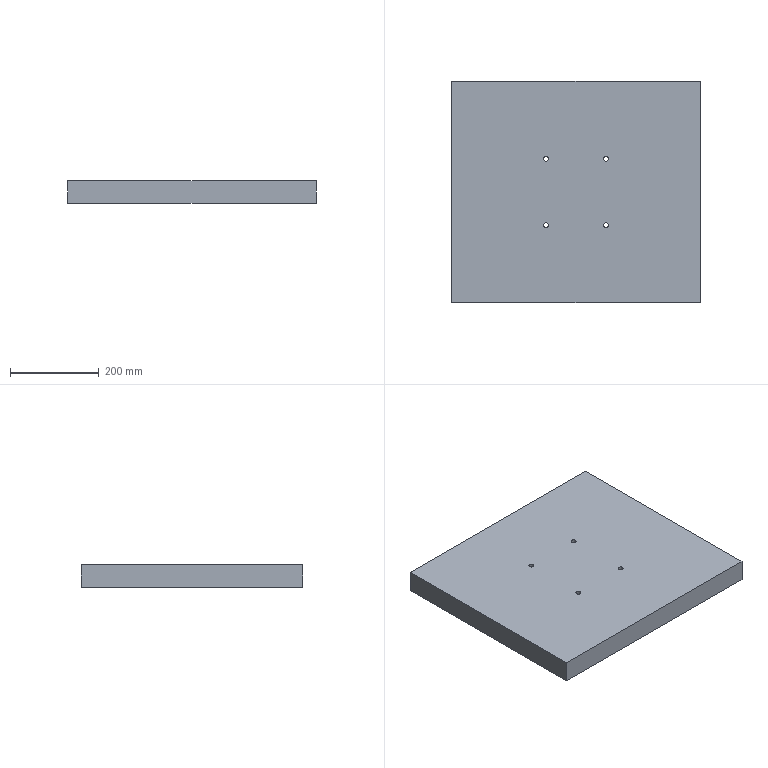Part | SolidWorks | features Extrusion 1, HoleWzd 1, ICE 1 | 1 solid | 22 faces | box 560 x 500 x 50 mm | volume 13976046 mm3 | cylinder 12 | plane 6 | cone 4 | commonest cylinder face diameters 11 x8 10.2 x4
STEP:
#1=CARTESIAN_POINT('',(-73.,-75.,0.));
#2=VERTEX_POINT('',#1);
#3=CARTESIAN_POINT('',(-62.,-75.,0.));
#4=VERTEX_POINT('',#3);
#5=CARTESIAN_POINT('',(-67.5,-75.,0.));
#6=DIRECTION('',(0.,0.,1.));
#7=DIRECTION('',(1.,0.,0.));
#8=AXIS2_PLACEMENT_3D('',#5,#6,#7);
#9=CIRCLE('',#8,5.5);
#10=EDGE_CURVE('',#2,#4,#9,.T.);
#11=ORIENTED_EDGE('',*,*,#10,.F.);
#12=CARTESIAN_POINT('',(-73.,-75.,50.));
#13=VERTEX_POINT('',#12);
#14=CARTESIAN_POINT('',(-73.,-75.,0.));
#15=DIRECTION('',(0.,0.,1.));
#16=VECTOR('',#15,1000.);
#17=LINE('',#14,#16);
#18=EDGE_CURVE('',#2,#13,#17,.T.);
#19=ORIENTED_EDGE('',*,*,#18,.T.);
#20=CARTESIAN_POINT('',(-62.,-75.,50.));
#21=VERTEX_POINT('',#20);
#22=CARTESIAN_POINT('',(-67.5,-75.,50.));
#23=DIRECTION('',(0.,0.,1.));
#24=DIRECTION('',(1.,0.,0.));
#25=AXIS2_PLACEMENT_3D('',#22,#23,#24);
#26=CIRCLE('',#25,5.5);
#27=EDGE_CURVE('',#13,#21,#26,.T.);
#28=ORIENTED_EDGE('',*,*,#27,.T.);
#29=CARTESIAN_POINT('',(-62.,-75.,0.));
#30=DIRECTION('',(0.,0.,1.));
#31=VECTOR('',#30,1000.);
#32=LINE('',#29,#31);
#33=EDGE_CURVE('',#4,#21,#32,.T.);
#34=ORIENTED_EDGE('',*,*,#33,.F.);
#35=EDGE_LOOP('',(#11,#19,#28,#34));
#36=FACE_OUTER_BOUND('',#35,.T.);
#37=CARTESIAN_POINT('',(-67.5,-75.,0.));
#38=DIRECTION('',(0.,0.,1.));
#39=DIRECTION('',(1.,0.,0.));
#40=AXIS2_PLACEMENT_3D('',#37,#38,#39);
#41=CYLINDRICAL_SURFACE('',#40,5.5);
#42=ADVANCED_FACE('',(#36),#41,.F.);
#43=CARTESIAN_POINT('',(62.,-75.,0.));
#44=VERTEX_POINT('',#43);
#45=CARTESIAN_POINT('',(73.,-75.,0.));
#46=VERTEX_POINT('',#45);
#47=CARTESIAN_POINT('',(67.5,-75.,0.));
#48=DIRECTION('',(0.,0.,1.));
#49=DIRECTION('',(1.,0.,0.));
#50=AXIS2_PLACEMENT_3D('',#47,#48,#49);
#51=CIRCLE('',#50,5.5);
#52=EDGE_CURVE('',#44,#46,#51,.T.);
#53=ORIENTED_EDGE('',*,*,#52,.F.);
#54=CARTESIAN_POINT('',(62.,-75.,50.));
#55=VERTEX_POINT('',#54);
#56=CARTESIAN_POINT('',(62.,-75.,0.));
#57=DIRECTION('',(0.,0.,1.));
#58=VECTOR('',#57,1000.);
#59=LINE('',#56,#58);
#60=EDGE_CURVE('',#44,#55,#59,.T.);
#61=ORIENTED_EDGE('',*,*,#60,.T.);
#62=CARTESIAN_POINT('',(73.,-75.,50.));
#63=VERTEX_POINT('',#62);
#64=CARTESIAN_POINT('',(67.5,-75.,50.));
#65=DIRECTION('',(0.,0.,1.));
#66=DIRECTION('',(1.,0.,0.));
#67=AXIS2_PLACEMENT_3D('',#64,#65,#66);
#68=CIRCLE('',#67,5.5);
#69=EDGE_CURVE('',#55,#63,#68,.T.);
#70=ORIENTED_EDGE('',*,*,#69,.T.);
#71=CARTESIAN_POINT('',(73.,-75.,0.));
#72=DIRECTION('',(0.,0.,1.));
#73=VECTOR('',#72,1000.);
#74=LINE('',#71,#73);
#75=EDGE_CURVE('',#46,#63,#74,.T.);
#76=ORIENTED_EDGE('',*,*,#75,.F.);
#77=EDGE_LOOP('',(#53,#61,#70,#76));
#78=FACE_OUTER_BOUND('',#77,.T.);
#79=CARTESIAN_POINT('',(67.5,-75.,0.));
#80=DIRECTION('',(0.,0.,1.));
#81=DIRECTION('',(1.,0.,0.));
#82=AXIS2_PLACEMENT_3D('',#79,#80,#81);
#83=CYLINDRICAL_SURFACE('',#82,5.5);
#84=ADVANCED_FACE('',(#78),#83,.F.);
#85=CARTESIAN_POINT('',(62.,75.,0.));
#86=VERTEX_POINT('',#85);
#87=CARTESIAN_POINT('',(73.,75.,0.));
#88=VERTEX_POINT('',#87);
#89=CARTESIAN_POINT('',(67.5,75.,0.));
#90=DIRECTION('',(0.,0.,1.));
#91=DIRECTION('',(1.,0.,0.));
#92=AXIS2_PLACEMENT_3D('',#89,#90,#91);
#93=CIRCLE('',#92,5.5);
#94=EDGE_CURVE('',#86,#88,#93,.T.);
#95=ORIENTED_EDGE('',*,*,#94,.F.);
#96=CARTESIAN_POINT('',(62.,75.,50.));
#97=VERTEX_POINT('',#96);
#98=CARTESIAN_POINT('',(62.,75.,0.));
#99=DIRECTION('',(0.,0.,1.));
#100=VECTOR('',#99,1000.);
#101=LINE('',#98,#100);
#102=EDGE_CURVE('',#86,#97,#101,.T.);
#103=ORIENTED_EDGE('',*,*,#102,.T.);
#104=CARTESIAN_POINT('',(73.,75.,50.));
#105=VERTEX_POINT('',#104);
#106=CARTESIAN_POINT('',(67.5,75.,50.));
#107=DIRECTION('',(0.,0.,1.));
#108=DIRECTION('',(1.,0.,0.));
#109=AXIS2_PLACEMENT_3D('',#106,#107,#108);
#110=CIRCLE('',#109,5.5);
#111=EDGE_CURVE('',#97,#105,#110,.T.);
#112=ORIENTED_EDGE('',*,*,#111,.T.);
#113=CARTESIAN_POINT('',(73.,75.,0.));
#114=DIRECTION('',(0.,0.,1.));
#115=VECTOR('',#114,1000.);
#116=LINE('',#113,#115);
#117=EDGE_CURVE('',#88,#105,#116,.T.);
#118=ORIENTED_EDGE('',*,*,#117,.F.);
#119=EDGE_LOOP('',(#95,#103,#112,#118));
#120=FACE_OUTER_BOUND('',#119,.T.);
#121=CARTESIAN_POINT('',(67.5,75.,0.));
#122=DIRECTION('',(0.,0.,1.));
#123=DIRECTION('',(1.,0.,0.));
#124=AXIS2_PLACEMENT_3D('',#121,#122,#123);
#125=CYLINDRICAL_SURFACE('',#124,5.5);
#126=ADVANCED_FACE('',(#120),#125,.F.);
#127=CARTESIAN_POINT('',(-73.,75.,0.));
#128=VERTEX_POINT('',#127);
#129=CARTESIAN_POINT('',(-62.,75.,0.));
#130=VERTEX_POINT('',#129);
#131=CARTESIAN_POINT('',(-67.5,75.,0.));
#132=DIRECTION('',(0.,0.,1.));
#133=DIRECTION('',(1.,0.,0.));
#134=AXIS2_PLACEMENT_3D('',#131,#132,#133);
#135=CIRCLE('',#134,5.5);
#136=EDGE_CURVE('',#128,#130,#135,.T.);
#137=ORIENTED_EDGE('',*,*,#136,.F.);
#138=CARTESIAN_POINT('',(-73.,75.,50.));
#139=VERTEX_POINT('',#138);
#140=CARTESIAN_POINT('',(-73.,75.,0.));
#141=DIRECTION('',(0.,0.,1.));
#142=VECTOR('',#141,1000.);
#143=LINE('',#140,#142);
#144=EDGE_CURVE('',#128,#139,#143,.T.);
#145=ORIENTED_EDGE('',*,*,#144,.T.);
#146=CARTESIAN_POINT('',(-62.,75.,50.));
#147=VERTEX_POINT('',#146);
#148=CARTESIAN_POINT('',(-67.5,75.,50.));
#149=DIRECTION('',(0.,0.,1.));
#150=DIRECTION('',(1.,0.,0.));
#151=AXIS2_PLACEMENT_3D('',#148,#149,#150);
#152=CIRCLE('',#151,5.5);
#153=EDGE_CURVE('',#139,#147,#152,.T.);
#154=ORIENTED_EDGE('',*,*,#153,.T.);
#155=CARTESIAN_POINT('',(-62.,75.,0.));
#156=DIRECTION('',(0.,0.,1.));
#157=VECTOR('',#156,1000.);
#158=LINE('',#155,#157);
#159=EDGE_CURVE('',#130,#147,#158,.T.);
#160=ORIENTED_EDGE('',*,*,#159,.F.);
#161=EDGE_LOOP('',(#137,#145,#154,#160));
#162=FACE_OUTER_BOUND('',#161,.T.);
#163=CARTESIAN_POINT('',(-67.5,75.,0.));
#164=DIRECTION('',(0.,0.,1.));
#165=DIRECTION('',(1.,0.,0.));
#166=AXIS2_PLACEMENT_3D('',#163,#164,#165);
#167=CYLINDRICAL_SURFACE('',#166,5.5);
#168=ADVANCED_FACE('',(#162),#167,.F.);
#169=CARTESIAN_POINT('',(-160.,220.75,19.9));
#170=VERTEX_POINT('',#169);
#171=CARTESIAN_POINT('',(-160.,220.75,30.1));
#172=VERTEX_POINT('',#171);
#173=CARTESIAN_POINT('',(-160.,220.75,25.));
#174=DIRECTION('',(0.,1.,0.));
#175=DIRECTION('',(0.,0.,1.));
#176=AXIS2_PLACEMENT_3D('',#173,#174,#175);
#177=CIRCLE('',#176,5.1);
#178=EDGE_CURVE('',#170,#172,#177,.T.);
#179=ORIENTED_EDGE('',*,*,#178,.F.);
#180=CARTESIAN_POINT('',(-160.,250.,19.9));
#181=VERTEX_POINT('',#180);
#182=CARTESIAN_POINT('',(-160.,250.,19.9));
#183=DIRECTION('',(0.,1.,0.));
#184=VECTOR('',#183,1000.);
#185=LINE('',#182,#184);
#186=EDGE_CURVE('',#170,#181,#185,.T.);
#187=ORIENTED_EDGE('',*,*,#186,.T.);
#188=CARTESIAN_POINT('',(-160.,250.,30.1));
#189=VERTEX_POINT('',#188);
#190=CARTESIAN_POINT('',(-160.,250.,25.));
#191=DIRECTION('',(0.,1.,0.));
#192=DIRECTION('',(0.,0.,1.));
#193=AXIS2_PLACEMENT_3D('',#190,#191,#192);
#194=CIRCLE('',#193,5.1);
#195=EDGE_CURVE('',#181,#189,#194,.T.);
#196=ORIENTED_EDGE('',*,*,#195,.T.);
#197=CARTESIAN_POINT('',(-160.,250.,30.1));
#198=DIRECTION('',(0.,1.,0.));
#199=VECTOR('',#198,1000.);
#200=LINE('',#197,#199);
#201=EDGE_CURVE('',#172,#189,#200,.T.);
#202=ORIENTED_EDGE('',*,*,#201,.F.);
#203=EDGE_LOOP('',(#179,#187,#196,#202));
#204=FACE_OUTER_BOUND('',#203,.T.);
#205=CARTESIAN_POINT('',(-160.,250.,25.));
#206=DIRECTION('',(0.,1.,0.));
#207=DIRECTION('',(0.,0.,1.));
#208=AXIS2_PLACEMENT_3D('',#205,#206,#207);
#209=CYLINDRICAL_SURFACE('',#208,5.1);
#210=ADVANCED_FACE('',(#204),#209,.F.);
#211=CARTESIAN_POINT('',(-160.,217.686,25.));
#212=VERTEX_POINT('',#211);
#213=CARTESIAN_POINT('',(-160.,220.75,30.1));
#214=DIRECTION('',(0.,0.515,0.8572));
#215=VECTOR('',#214,1000.);
#216=LINE('',#213,#215);
#217=EDGE_CURVE('',#212,#172,#216,.T.);
#218=ORIENTED_EDGE('',*,*,#217,.F.);
#219=CARTESIAN_POINT('',(-160.,220.75,19.9));
#220=DIRECTION('',(0.,0.515,-0.8572));
#221=VECTOR('',#220,1000.);
#222=LINE('',#219,#221);
#223=EDGE_CURVE('',#212,#170,#222,.T.);
#224=ORIENTED_EDGE('',*,*,#223,.T.);
#225=ORIENTED_EDGE('',*,*,#178,.T.);
#226=EDGE_LOOP('',(#218,#224,#225));
#227=FACE_OUTER_BOUND('',#226,.T.);
#228=CARTESIAN_POINT('',(-160.,220.75,25.));
#229=DIRECTION('',(0.,1.,0.));
#230=DIRECTION('',(0.,0.,1.));
#231=AXIS2_PLACEMENT_3D('',#228,#229,#230);
#232=CONICAL_SURFACE('',#231,5.1,1.03);
#233=ADVANCED_FACE('',(#227),#232,.F.);
#234=CARTESIAN_POINT('',(160.,220.75,19.9));
#235=VERTEX_POINT('',#234);
#236=CARTESIAN_POINT('',(160.,220.75,30.1));
#237=VERTEX_POINT('',#236);
#238=CARTESIAN_POINT('',(160.,220.75,25.));
#239=DIRECTION('',(0.,1.,0.));
#240=DIRECTION('',(0.,0.,1.));
#241=AXIS2_PLACEMENT_3D('',#238,#239,#240);
#242=CIRCLE('',#241,5.1);
#243=EDGE_CURVE('',#235,#237,#242,.T.);
#244=ORIENTED_EDGE('',*,*,#243,.F.);
#245=CARTESIAN_POINT('',(160.,250.,19.9));
#246=VERTEX_POINT('',#245);
#247=CARTESIAN_POINT('',(160.,250.,19.9));
#248=DIRECTION('',(0.,1.,0.));
#249=VECTOR('',#248,1000.);
#250=LINE('',#247,#249);
#251=EDGE_CURVE('',#235,#246,#250,.T.);
#252=ORIENTED_EDGE('',*,*,#251,.T.);
#253=CARTESIAN_POINT('',(160.,250.,30.1));
#254=VERTEX_POINT('',#253);
#255=CARTESIAN_POINT('',(160.,250.,25.));
#256=DIRECTION('',(0.,1.,0.));
#257=DIRECTION('',(0.,0.,1.));
#258=AXIS2_PLACEMENT_3D('',#255,#256,#257);
#259=CIRCLE('',#258,5.1);
#260=EDGE_CURVE('',#246,#254,#259,.T.);
#261=ORIENTED_EDGE('',*,*,#260,.T.);
#262=CARTESIAN_POINT('',(160.,250.,30.1));
#263=DIRECTION('',(0.,1.,0.));
#264=VECTOR('',#263,1000.);
#265=LINE('',#262,#264);
#266=EDGE_CURVE('',#237,#254,#265,.T.);
#267=ORIENTED_EDGE('',*,*,#266,.F.);
#268=EDGE_LOOP('',(#244,#252,#261,#267));
#269=FACE_OUTER_BOUND('',#268,.T.);
#270=CARTESIAN_POINT('',(160.,250.,25.));
#271=DIRECTION('',(0.,1.,0.));
#272=DIRECTION('',(0.,0.,1.));
#273=AXIS2_PLACEMENT_3D('',#270,#271,#272);
#274=CYLINDRICAL_SURFACE('',#273,5.1);
#275=ADVANCED_FACE('',(#269),#274,.F.);
#276=CARTESIAN_POINT('',(160.,217.686,25.));
#277=VERTEX_POINT('',#276);
#278=CARTESIAN_POINT('',(160.,220.75,30.1));
#279=DIRECTION('',(0.,0.515,0.8572));
#280=VECTOR('',#279,1000.);
#281=LINE('',#278,#280);
#282=EDGE_CURVE('',#277,#237,#281,.T.);
#283=ORIENTED_EDGE('',*,*,#282,.F.);
#284=CARTESIAN_POINT('',(160.,220.75,19.9));
#285=DIRECTION('',(0.,0.515,-0.8572));
#286=VECTOR('',#285,1000.);
#287=LINE('',#284,#286);
#288=EDGE_CURVE('',#277,#235,#287,.T.);
#289=ORIENTED_EDGE('',*,*,#288,.T.);
#290=ORIENTED_EDGE('',*,*,#243,.T.);
#291=EDGE_LOOP('',(#283,#289,#290));
#292=FACE_OUTER_BOUND('',#291,.T.);
#293=CARTESIAN_POINT('',(160.,220.75,25.));
#294=DIRECTION('',(0.,1.,0.));
#295=DIRECTION('',(0.,0.,1.));
#296=AXIS2_PLACEMENT_3D('',#293,#294,#295);
#297=CONICAL_SURFACE('',#296,5.1,1.03);
#298=ADVANCED_FACE('',(#292),#297,.F.);
#299=CARTESIAN_POINT('',(-280.,250.,0.));
#300=VERTEX_POINT('',#299);
#301=CARTESIAN_POINT('',(-280.,-250.,0.));
#302=VERTEX_POINT('',#301);
#303=CARTESIAN_POINT('',(-280.,250.,0.));
#304=DIRECTION('',(0.,-1.,0.));
#305=VECTOR('',#304,1000.);
#306=LINE('',#303,#305);
#307=EDGE_CURVE('',#300,#302,#306,.T.);
#308=ORIENTED_EDGE('',*,*,#307,.T.);
#309=CARTESIAN_POINT('',(-280.,-250.,50.));
#310=VERTEX_POINT('',#309);
#311=CARTESIAN_POINT('',(-280.,-250.,50.));
#312=DIRECTION('',(0.,0.,-1.));
#313=VECTOR('',#312,1000.);
#314=LINE('',#311,#313);
#315=EDGE_CURVE('',#310,#302,#314,.T.);
#316=ORIENTED_EDGE('',*,*,#315,.F.);
#317=CARTESIAN_POINT('',(-280.,250.,50.));
#318=VERTEX_POINT('',#317);
#319=CARTESIAN_POINT('',(-280.,250.,50.));
#320=DIRECTION('',(0.,-1.,0.));
#321=VECTOR('',#320,1000.);
#322=LINE('',#319,#321);
#323=EDGE_CURVE('',#318,#310,#322,.T.);
#324=ORIENTED_EDGE('',*,*,#323,.F.);
#325=CARTESIAN_POINT('',(-280.,250.,50.));
#326=DIRECTION('',(0.,0.,-1.));
#327=VECTOR('',#326,1000.);
#328=LINE('',#325,#327);
#329=EDGE_CURVE('',#318,#300,#328,.T.);
#330=ORIENTED_EDGE('',*,*,#329,.T.);
#331=EDGE_LOOP('',(#308,#316,#324,#330));
#332=FACE_OUTER_BOUND('',#331,.T.);
#333=CARTESIAN_POINT('',(-280.,250.,50.));
#334=DIRECTION('',(1.,0.,0.));
#335=DIRECTION('',(0.,1.,0.));
#336=AXIS2_PLACEMENT_3D('',#333,#334,#335);
#337=PLANE('',#336);
#338=ADVANCED_FACE('',(#332),#337,.F.);
#339=CARTESIAN_POINT('',(280.,-250.,0.));
#340=VERTEX_POINT('',#339);
#341=CARTESIAN_POINT('',(280.,-250.,0.));
#342=DIRECTION('',(1.,0.,0.));
#343=VECTOR('',#342,1000.);
#344=LINE('',#341,#343);
#345=EDGE_CURVE('',#302,#340,#344,.T.);
#346=ORIENTED_EDGE('',*,*,#345,.T.);
#347=CARTESIAN_POINT('',(280.,-250.,50.));
#348=VERTEX_POINT('',#347);
#349=CARTESIAN_POINT('',(280.,-250.,50.));
#350=DIRECTION('',(0.,0.,-1.));
#351=VECTOR('',#350,1000.);
#352=LINE('',#349,#351);
#353=EDGE_CURVE('',#348,#340,#352,.T.);
#354=ORIENTED_EDGE('',*,*,#353,.F.);
#355=CARTESIAN_POINT('',(280.,-250.,50.));
#356=DIRECTION('',(1.,0.,0.));
#357=VECTOR('',#356,1000.);
#358=LINE('',#355,#357);
#359=EDGE_CURVE('',#310,#348,#358,.T.);
#360=ORIENTED_EDGE('',*,*,#359,.F.);
#361=ORIENTED_EDGE('',*,*,#315,.T.);
#362=EDGE_LOOP('',(#346,#354,#360,#361));
#363=FACE_OUTER_BOUND('',#362,.T.);
#364=CARTESIAN_POINT('',(280.,-250.,50.));
#365=DIRECTION('',(0.,1.,0.));
#366=DIRECTION('',(-1.,0.,0.));
#367=AXIS2_PLACEMENT_3D('',#364,#365,#366);
#368=PLANE('',#367);
#369=ADVANCED_FACE('',(#363),#368,.F.);
#370=CARTESIAN_POINT('',(280.,250.,0.));
#371=VERTEX_POINT('',#370);
#372=CARTESIAN_POINT('',(280.,250.,0.));
#373=DIRECTION('',(0.,1.,0.));
#374=VECTOR('',#373,1000.);
#375=LINE('',#372,#374);
#376=EDGE_CURVE('',#340,#371,#375,.T.);
#377=ORIENTED_EDGE('',*,*,#376,.T.);
#378=CARTESIAN_POINT('',(280.,250.,50.));
#379=VERTEX_POINT('',#378);
#380=CARTESIAN_POINT('',(280.,250.,50.));
#381=DIRECTION('',(0.,0.,-1.));
#382=VECTOR('',#381,1000.);
#383=LINE('',#380,#382);
#384=EDGE_CURVE('',#379,#371,#383,.T.);
#385=ORIENTED_EDGE('',*,*,#384,.F.);
#386=CARTESIAN_POINT('',(280.,250.,50.));
#387=DIRECTION('',(0.,1.,0.));
#388=VECTOR('',#387,1000.);
#389=LINE('',#386,#388);
#390=EDGE_CURVE('',#348,#379,#389,.T.);
#391=ORIENTED_EDGE('',*,*,#390,.F.);
#392=ORIENTED_EDGE('',*,*,#353,.T.);
#393=EDGE_LOOP('',(#377,#385,#391,#392));
#394=FACE_OUTER_BOUND('',#393,.T.);
#395=CARTESIAN_POINT('',(280.,250.,50.));
#396=DIRECTION('',(-1.,0.,0.));
#397=DIRECTION('',(0.,-1.,0.));
#398=AXIS2_PLACEMENT_3D('',#395,#396,#397);
#399=PLANE('',#398);
#400=ADVANCED_FACE('',(#394),#399,.F.);
#401=CARTESIAN_POINT('',(-160.,250.,25.));
#402=DIRECTION('',(0.,1.,0.));
#403=DIRECTION('',(0.,0.,1.));
#404=AXIS2_PLACEMENT_3D('',#401,#402,#403);
#405=CIRCLE('',#404,5.1);
#406=EDGE_CURVE('',#189,#181,#405,.T.);
#407=ORIENTED_EDGE('',*,*,#406,.F.);
#408=ORIENTED_EDGE('',*,*,#195,.F.);
#409=EDGE_LOOP('',(#407,#408));
#410=FACE_BOUND('',#409,.T.);
#411=CARTESIAN_POINT('',(160.,250.,25.));
#412=DIRECTION('',(0.,1.,0.));
#413=DIRECTION('',(0.,0.,1.));
#414=AXIS2_PLACEMENT_3D('',#411,#412,#413);
#415=CIRCLE('',#414,5.1);
#416=EDGE_CURVE('',#254,#246,#415,.T.);
#417=ORIENTED_EDGE('',*,*,#416,.F.);
#418=ORIENTED_EDGE('',*,*,#260,.F.);
#419=EDGE_LOOP('',(#417,#418));
#420=FACE_BOUND('',#419,.T.);
#421=CARTESIAN_POINT('',(280.,250.,0.));
#422=DIRECTION('',(-1.,0.,0.));
#423=VECTOR('',#422,1000.);
#424=LINE('',#421,#423);
#425=EDGE_CURVE('',#371,#300,#424,.T.);
#426=ORIENTED_EDGE('',*,*,#425,.T.);
#427=ORIENTED_EDGE('',*,*,#329,.F.);
#428=CARTESIAN_POINT('',(280.,250.,50.));
#429=DIRECTION('',(-1.,0.,0.));
#430=VECTOR('',#429,1000.);
#431=LINE('',#428,#430);
#432=EDGE_CURVE('',#379,#318,#431,.T.);
#433=ORIENTED_EDGE('',*,*,#432,.F.);
#434=ORIENTED_EDGE('',*,*,#384,.T.);
#435=EDGE_LOOP('',(#426,#427,#433,#434));
#436=FACE_OUTER_BOUND('',#435,.T.);
#437=CARTESIAN_POINT('',(280.,250.,50.));
#438=DIRECTION('',(0.,-1.,0.));
#439=DIRECTION('',(1.,0.,0.));
#440=AXIS2_PLACEMENT_3D('',#437,#438,#439);
#441=PLANE('',#440);
#442=ADVANCED_FACE('',(#410,#420,#436),#441,.F.);
#443=CARTESIAN_POINT('',(-67.5,-75.,50.));
#444=DIRECTION('',(0.,0.,1.));
#445=DIRECTION('',(1.,0.,0.));
#446=AXIS2_PLACEMENT_3D('',#443,#444,#445);
#447=CIRCLE('',#446,5.5);
#448=EDGE_CURVE('',#21,#13,#447,.T.);
#449=ORIENTED_EDGE('',*,*,#448,.F.);
#450=ORIENTED_EDGE('',*,*,#27,.F.);
#451=EDGE_LOOP('',(#449,#450));
#452=FACE_BOUND('',#451,.T.);
#453=CARTESIAN_POINT('',(67.5,-75.,50.));
#454=DIRECTION('',(0.,0.,1.));
#455=DIRECTION('',(1.,0.,0.));
#456=AXIS2_PLACEMENT_3D('',#453,#454,#455);
#457=CIRCLE('',#456,5.5);
#458=EDGE_CURVE('',#63,#55,#457,.T.);
#459=ORIENTED_EDGE('',*,*,#458,.F.);
#460=ORIENTED_EDGE('',*,*,#69,.F.);
#461=EDGE_LOOP('',(#459,#460));
#462=FACE_BOUND('',#461,.T.);
#463=CARTESIAN_POINT('',(67.5,75.,50.));
#464=DIRECTION('',(0.,0.,1.));
#465=DIRECTION('',(1.,0.,0.));
#466=AXIS2_PLACEMENT_3D('',#463,#464,#465);
#467=CIRCLE('',#466,5.5);
#468=EDGE_CURVE('',#105,#97,#467,.T.);
#469=ORIENTED_EDGE('',*,*,#468,.F.);
#470=ORIENTED_EDGE('',*,*,#111,.F.);
#471=EDGE_LOOP('',(#469,#470));
#472=FACE_BOUND('',#471,.T.);
#473=CARTESIAN_POINT('',(-67.5,75.,50.));
#474=DIRECTION('',(0.,0.,1.));
#475=DIRECTION('',(1.,0.,0.));
#476=AXIS2_PLACEMENT_3D('',#473,#474,#475);
#477=CIRCLE('',#476,5.5);
#478=EDGE_CURVE('',#147,#139,#477,.T.);
#479=ORIENTED_EDGE('',*,*,#478,.F.);
#480=ORIENTED_EDGE('',*,*,#153,.F.);
#481=EDGE_LOOP('',(#479,#480));
#482=FACE_BOUND('',#481,.T.);
#483=ORIENTED_EDGE('',*,*,#323,.T.);
#484=ORIENTED_EDGE('',*,*,#359,.T.);
#485=ORIENTED_EDGE('',*,*,#390,.T.);
#486=ORIENTED_EDGE('',*,*,#432,.T.);
#487=EDGE_LOOP('',(#483,#484,#485,#486));
#488=FACE_OUTER_BOUND('',#487,.T.);
#489=CARTESIAN_POINT('',(0.,0.,50.));
#490=DIRECTION('',(0.,0.,-1.));
#491=DIRECTION('',(-1.,0.,0.));
#492=AXIS2_PLACEMENT_3D('',#489,#490,#491);
#493=PLANE('',#492);
#494=ADVANCED_FACE('',(#452,#462,#472,#482,#488),#493,.F.);
#495=CARTESIAN_POINT('',(-67.5,-75.,0.));
#496=DIRECTION('',(0.,0.,1.));
#497=DIRECTION('',(1.,0.,0.));
#498=AXIS2_PLACEMENT_3D('',#495,#496,#497);
#499=CIRCLE('',#498,5.5);
#500=EDGE_CURVE('',#4,#2,#499,.T.);
#501=ORIENTED_EDGE('',*,*,#500,.T.);
#502=ORIENTED_EDGE('',*,*,#10,.T.);
#503=EDGE_LOOP('',(#501,#502));
#504=FACE_BOUND('',#503,.T.);
#505=CARTESIAN_POINT('',(67.5,-75.,0.));
#506=DIRECTION('',(0.,0.,1.));
#507=DIRECTION('',(1.,0.,0.));
#508=AXIS2_PLACEMENT_3D('',#505,#506,#507);
#509=CIRCLE('',#508,5.5);
#510=EDGE_CURVE('',#46,#44,#509,.T.);
#511=ORIENTED_EDGE('',*,*,#510,.T.);
#512=ORIENTED_EDGE('',*,*,#52,.T.);
#513=EDGE_LOOP('',(#511,#512));
#514=FACE_BOUND('',#513,.T.);
#515=CARTESIAN_POINT('',(67.5,75.,0.));
#516=DIRECTION('',(0.,0.,1.));
#517=DIRECTION('',(1.,0.,0.));
#518=AXIS2_PLACEMENT_3D('',#515,#516,#517);
#519=CIRCLE('',#518,5.5);
#520=EDGE_CURVE('',#88,#86,#519,.T.);
#521=ORIENTED_EDGE('',*,*,#520,.T.);
#522=ORIENTED_EDGE('',*,*,#94,.T.);
#523=EDGE_LOOP('',(#521,#522));
#524=FACE_BOUND('',#523,.T.);
#525=CARTESIAN_POINT('',(-67.5,75.,0.));
#526=DIRECTION('',(0.,0.,1.));
#527=DIRECTION('',(1.,0.,0.));
#528=AXIS2_PLACEMENT_3D('',#525,#526,#527);
#529=CIRCLE('',#528,5.5);
#530=EDGE_CURVE('',#130,#128,#529,.T.);
#531=ORIENTED_EDGE('',*,*,#530,.T.);
#532=ORIENTED_EDGE('',*,*,#136,.T.);
#533=EDGE_LOOP('',(#531,#532));
#534=FACE_BOUND('',#533,.T.);
#535=ORIENTED_EDGE('',*,*,#307,.F.);
#536=ORIENTED_EDGE('',*,*,#425,.F.);
#537=ORIENTED_EDGE('',*,*,#376,.F.);
#538=ORIENTED_EDGE('',*,*,#345,.F.);
#539=EDGE_LOOP('',(#535,#536,#537,#538));
#540=FACE_OUTER_BOUND('',#539,.T.);
#541=CARTESIAN_POINT('',(0.,0.,0.));
#542=DIRECTION('',(0.,0.,-1.));
#543=DIRECTION('',(-1.,0.,0.));
#544=AXIS2_PLACEMENT_3D('',#541,#542,#543);
#545=PLANE('',#544);
#546=ADVANCED_FACE('',(#504,#514,#524,#534,#540),#545,.T.);
#547=ORIENTED_EDGE('',*,*,#288,.F.);
#548=ORIENTED_EDGE('',*,*,#282,.T.);
#549=CARTESIAN_POINT('',(160.,220.75,25.));
#550=DIRECTION('',(0.,1.,0.));
#551=DIRECTION('',(0.,0.,1.));
#552=AXIS2_PLACEMENT_3D('',#549,#550,#551);
#553=CIRCLE('',#552,5.1);
#554=EDGE_CURVE('',#237,#235,#553,.T.);
#555=ORIENTED_EDGE('',*,*,#554,.T.);
#556=EDGE_LOOP('',(#547,#548,#555));
#557=FACE_OUTER_BOUND('',#556,.T.);
#558=CARTESIAN_POINT('',(160.,220.75,25.));
#559=DIRECTION('',(0.,1.,0.));
#560=DIRECTION('',(0.,0.,1.));
#561=AXIS2_PLACEMENT_3D('',#558,#559,#560);
#562=CONICAL_SURFACE('',#561,5.1,1.03);
#563=ADVANCED_FACE('',(#557),#562,.F.);
#564=ORIENTED_EDGE('',*,*,#251,.F.);
#565=ORIENTED_EDGE('',*,*,#554,.F.);
#566=ORIENTED_EDGE('',*,*,#266,.T.);
#567=ORIENTED_EDGE('',*,*,#416,.T.);
#568=EDGE_LOOP('',(#564,#565,#566,#567));
#569=FACE_OUTER_BOUND('',#568,.T.);
#570=CARTESIAN_POINT('',(160.,250.,25.));
#571=DIRECTION('',(0.,1.,0.));
#572=DIRECTION('',(0.,0.,1.));
#573=AXIS2_PLACEMENT_3D('',#570,#571,#572);
#574=CYLINDRICAL_SURFACE('',#573,5.1);
#575=ADVANCED_FACE('',(#569),#574,.F.);
#576=ORIENTED_EDGE('',*,*,#223,.F.);
#577=ORIENTED_EDGE('',*,*,#217,.T.);
#578=CARTESIAN_POINT('',(-160.,220.75,25.));
#579=DIRECTION('',(0.,1.,0.));
#580=DIRECTION('',(0.,0.,1.));
#581=AXIS2_PLACEMENT_3D('',#578,#579,#580);
#582=CIRCLE('',#581,5.1);
#583=EDGE_CURVE('',#172,#170,#582,.T.);
#584=ORIENTED_EDGE('',*,*,#583,.T.);
#585=EDGE_LOOP('',(#576,#577,#584));
#586=FACE_OUTER_BOUND('',#585,.T.);
#587=CARTESIAN_POINT('',(-160.,220.75,25.));
#588=DIRECTION('',(0.,1.,0.));
#589=DIRECTION('',(0.,0.,1.));
#590=AXIS2_PLACEMENT_3D('',#587,#588,#589);
#591=CONICAL_SURFACE('',#590,5.1,1.03);
#592=ADVANCED_FACE('',(#586),#591,.F.);
#593=ORIENTED_EDGE('',*,*,#186,.F.);
#594=ORIENTED_EDGE('',*,*,#583,.F.);
#595=ORIENTED_EDGE('',*,*,#201,.T.);
#596=ORIENTED_EDGE('',*,*,#406,.T.);
#597=EDGE_LOOP('',(#593,#594,#595,#596));
#598=FACE_OUTER_BOUND('',#597,.T.);
#599=CARTESIAN_POINT('',(-160.,250.,25.));
#600=DIRECTION('',(0.,1.,0.));
#601=DIRECTION('',(0.,0.,1.));
#602=AXIS2_PLACEMENT_3D('',#599,#600,#601);
#603=CYLINDRICAL_SURFACE('',#602,5.1);
#604=ADVANCED_FACE('',(#598),#603,.F.);
#605=ORIENTED_EDGE('',*,*,#144,.F.);
#606=ORIENTED_EDGE('',*,*,#530,.F.);
#607=ORIENTED_EDGE('',*,*,#159,.T.);
#608=ORIENTED_EDGE('',*,*,#478,.T.);
#609=EDGE_LOOP('',(#605,#606,#607,#608));
#610=FACE_OUTER_BOUND('',#609,.T.);
#611=CARTESIAN_POINT('',(-67.5,75.,0.));
#612=DIRECTION('',(0.,0.,1.));
#613=DIRECTION('',(1.,0.,0.));
#614=AXIS2_PLACEMENT_3D('',#611,#612,#613);
#615=CYLINDRICAL_SURFACE('',#614,5.5);
#616=ADVANCED_FACE('',(#610),#615,.F.);
#617=ORIENTED_EDGE('',*,*,#102,.F.);
#618=ORIENTED_EDGE('',*,*,#520,.F.);
#619=ORIENTED_EDGE('',*,*,#117,.T.);
#620=ORIENTED_EDGE('',*,*,#468,.T.);
#621=EDGE_LOOP('',(#617,#618,#619,#620));
#622=FACE_OUTER_BOUND('',#621,.T.);
#623=CARTESIAN_POINT('',(67.5,75.,0.));
#624=DIRECTION('',(0.,0.,1.));
#625=DIRECTION('',(1.,0.,0.));
#626=AXIS2_PLACEMENT_3D('',#623,#624,#625);
#627=CYLINDRICAL_SURFACE('',#626,5.5);
#628=ADVANCED_FACE('',(#622),#627,.F.);
#629=ORIENTED_EDGE('',*,*,#60,.F.);
#630=ORIENTED_EDGE('',*,*,#510,.F.);
#631=ORIENTED_EDGE('',*,*,#75,.T.);
#632=ORIENTED_EDGE('',*,*,#458,.T.);
#633=EDGE_LOOP('',(#629,#630,#631,#632));
#634=FACE_OUTER_BOUND('',#633,.T.);
#635=CARTESIAN_POINT('',(67.5,-75.,0.));
#636=DIRECTION('',(0.,0.,1.));
#637=DIRECTION('',(1.,0.,0.));
#638=AXIS2_PLACEMENT_3D('',#635,#636,#637);
#639=CYLINDRICAL_SURFACE('',#638,5.5);
#640=ADVANCED_FACE('',(#634),#639,.F.);
#641=ORIENTED_EDGE('',*,*,#18,.F.);
#642=ORIENTED_EDGE('',*,*,#500,.F.);
#643=ORIENTED_EDGE('',*,*,#33,.T.);
#644=ORIENTED_EDGE('',*,*,#448,.T.);
#645=EDGE_LOOP('',(#641,#642,#643,#644));
#646=FACE_OUTER_BOUND('',#645,.T.);
#647=CARTESIAN_POINT('',(-67.5,-75.,0.));
#648=DIRECTION('',(0.,0.,1.));
#649=DIRECTION('',(1.,0.,0.));
#650=AXIS2_PLACEMENT_3D('',#647,#648,#649);
#651=CYLINDRICAL_SURFACE('',#650,5.5);
#652=ADVANCED_FACE('',(#646),#651,.F.);
#653=CLOSED_SHELL('',(#42,#84,#126,#168,#210,#233,#275,#298,#338,#369,#400,#442,#494,#546,#563,#575,#592,#604,#616,#628,#640,#652));
#654=MANIFOLD_SOLID_BREP('',#653);
#655=CARTESIAN_POINT('',(0.,0.,0.));
#656=DIRECTION('',(0.,0.,1.));
#657=DIRECTION('',(1.,0.,0.));
#658=AXIS2_PLACEMENT_3D('',#655,#656,#657);
#659=(LENGTH_UNIT()NAMED_UNIT(*)SI_UNIT(.MILLI.,.METRE.));
#660=UNCERTAINTY_MEASURE_WITH_UNIT(LENGTH_MEASURE(0.00001),#659,'','');
#661=(NAMED_UNIT(*)PLANE_ANGLE_UNIT()SI_UNIT($,.RADIAN.));
#662=(NAMED_UNIT(*)SI_UNIT($,.STERADIAN.)SOLID_ANGLE_UNIT());
#663=(GEOMETRIC_REPRESENTATION_CONTEXT(3)GLOBAL_UNCERTAINTY_ASSIGNED_CONTEXT((#660))GLOBAL_UNIT_ASSIGNED_CONTEXT((#659,#661,#662))REPRESENTATION_CONTEXT('',''));
#664=ADVANCED_BREP_SHAPE_REPRESENTATION('',(#654,#658),#663);